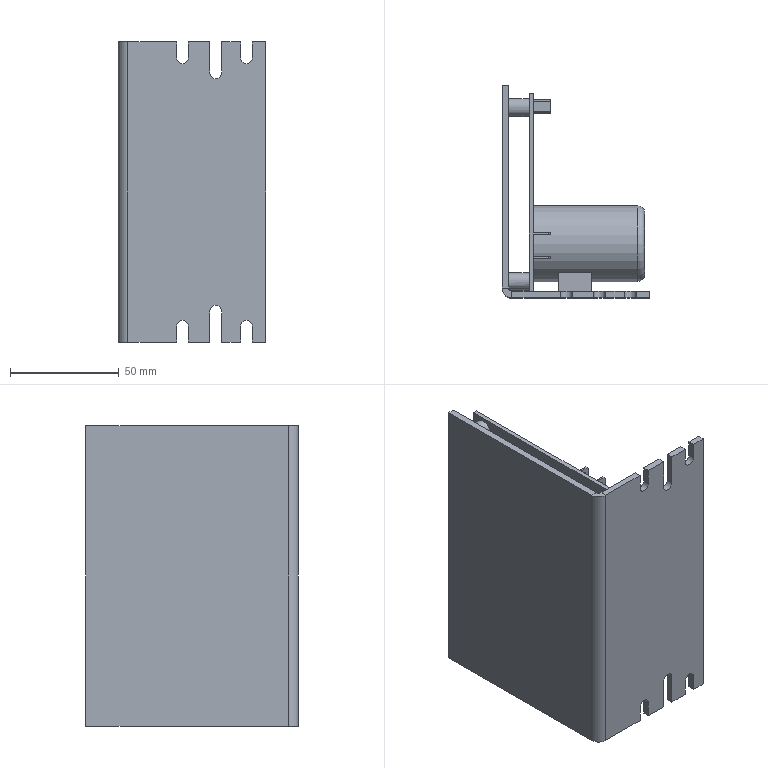Part | STEP file | ZY03WYF | 1 solid | 142 faces | box 68 x 97.5 x 138 mm | volume 146420 mm3 | plane 124 | cylinder 17 | torus 1 | commonest cylinder face diameters 5.4 x6 2 x4 8 x4 3 x1 9 x1 35 x1